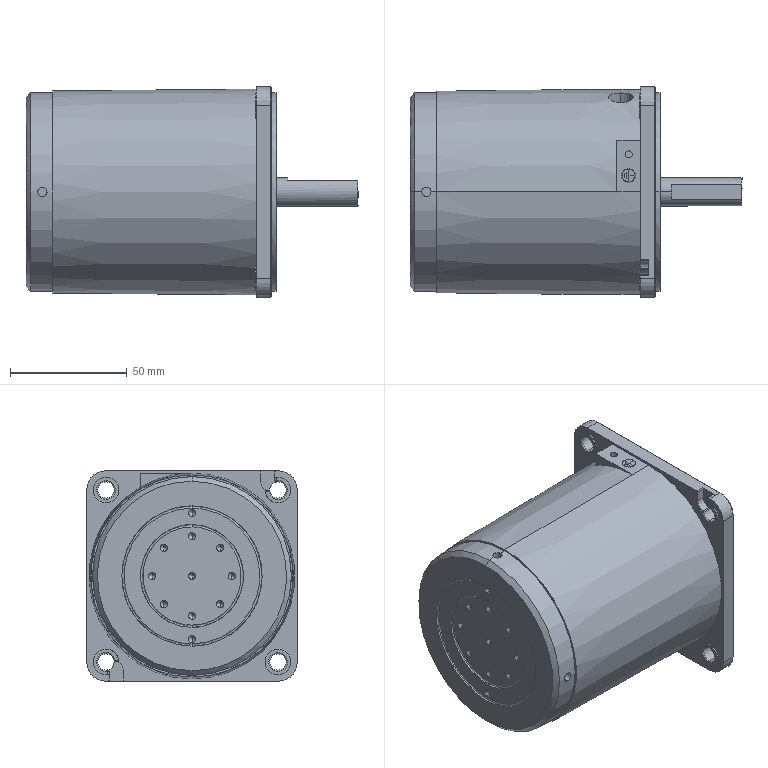Part | STEP file | ADMI9201SOYF_22_1 | 1 solid | 179 faces | box 142 x 90 x 90 mm | volume 645514 mm3 | cylinder 65 | plane 60 | spline 28 | cone 26 | commonest cylinder face diameters 1 x11 7 x10 11 x10 4 x8 15 x4 16 x4